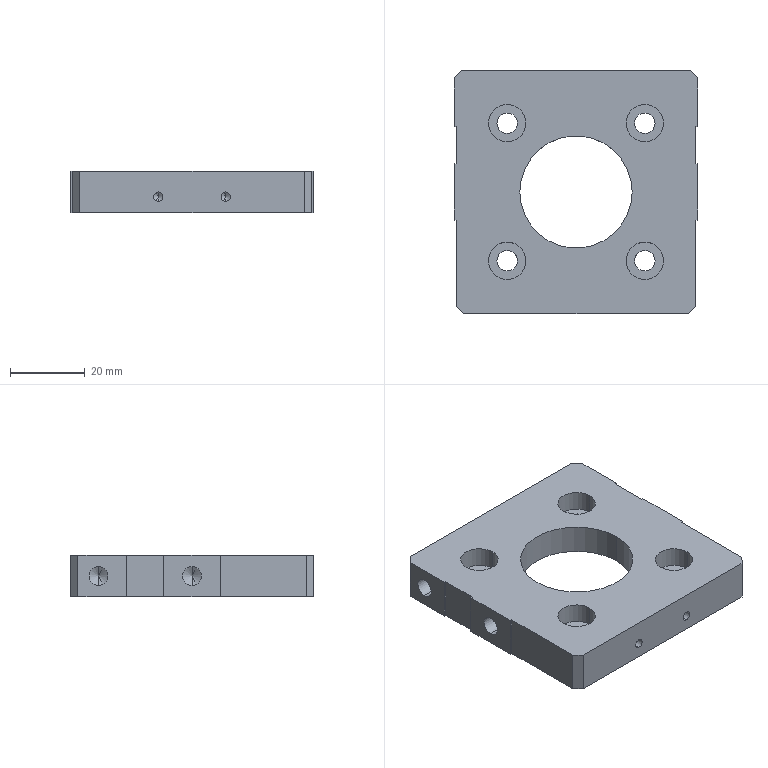Part | SolidWorks | features HoleWzd 5, ICE 4, Chamfer 1, Extrusion 1, MirrorPattern 1 | 1 solid | 79 faces | box 65 x 65 x 11 mm | volume 33278 mm3 | cylinder 36 | plane 27 | cone 16 | commonest cylinder face diameters 2.5 x8 5 x8 5.5 x8 10 x8 30 x2 40.1 x2